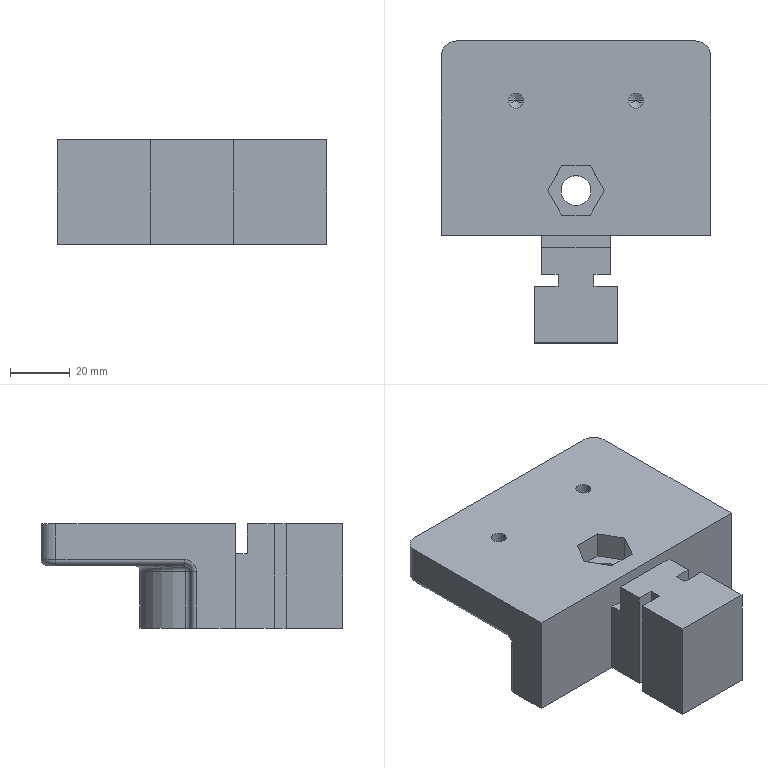Part | SolidWorks | features ICE 3, Cut 1, Extrusion 1, Fillet 1, HoleWzd 1 | 1 solid | 59 faces | box 90 x 101 x 35 mm | volume 144752 mm3 | plane 30 | cylinder 18 | torus 5 | cone 4 | sphere 2 | commonest cylinder face diameters 4 x9 5 x4 10 x4 34 x1